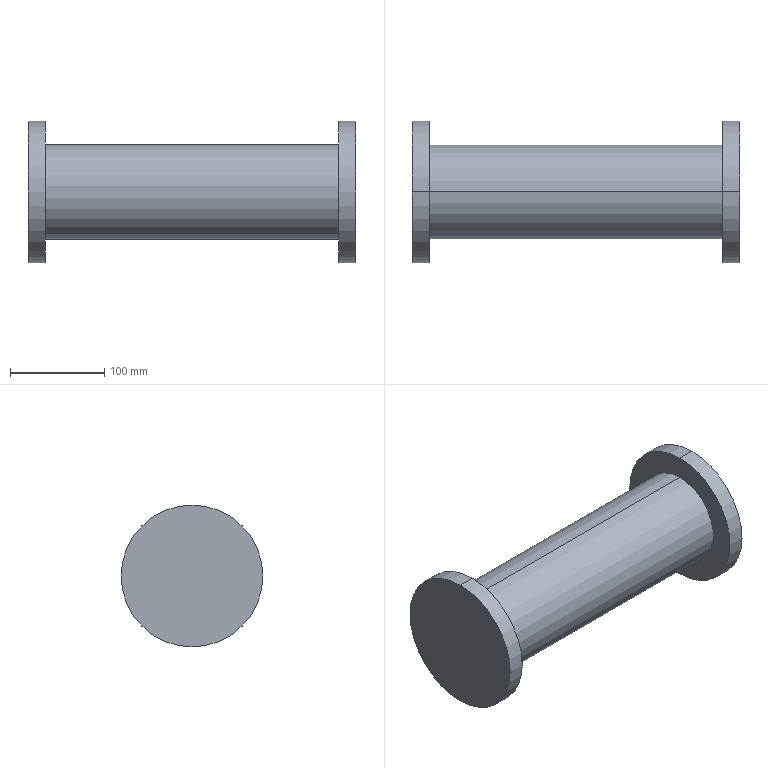Part | SolidWorks | features ICE 2, Extrusion 1 | 1 solid | 10 faces | box 347 x 150 x 150 mm | volume 3078761 mm3 | cylinder 6 | plane 4 | commonest cylinder face diameters 150 x4 100 x2
STEP:
#1=CARTESIAN_POINT('',(-329.,0.,-75.));
#2=VERTEX_POINT('',#1);
#3=CARTESIAN_POINT('',(-329.,0.,75.));
#4=VERTEX_POINT('',#3);
#5=CARTESIAN_POINT('',(-329.,0.,0.));
#6=DIRECTION('',(1.,0.,0.));
#7=DIRECTION('',(0.,0.,-1.));
#8=AXIS2_PLACEMENT_3D('',#5,#6,#7);
#9=CIRCLE('',#8,75.);
#10=EDGE_CURVE('',#2,#4,#9,.T.);
#11=ORIENTED_EDGE('',*,*,#10,.T.);
#12=CARTESIAN_POINT('',(-311.,0.,75.));
#13=VERTEX_POINT('',#12);
#14=CARTESIAN_POINT('',(-329.,0.,75.));
#15=DIRECTION('',(1.,0.,0.));
#16=VECTOR('',#15,1000.);
#17=LINE('',#14,#16);
#18=EDGE_CURVE('',#4,#13,#17,.T.);
#19=ORIENTED_EDGE('',*,*,#18,.T.);
#20=CARTESIAN_POINT('',(-311.,0.,-75.));
#21=VERTEX_POINT('',#20);
#22=CARTESIAN_POINT('',(-311.,0.,0.));
#23=DIRECTION('',(1.,0.,0.));
#24=DIRECTION('',(0.,0.,-1.));
#25=AXIS2_PLACEMENT_3D('',#22,#23,#24);
#26=CIRCLE('',#25,75.);
#27=EDGE_CURVE('',#21,#13,#26,.T.);
#28=ORIENTED_EDGE('',*,*,#27,.F.);
#29=CARTESIAN_POINT('',(-329.,0.,-75.));
#30=DIRECTION('',(1.,0.,0.));
#31=VECTOR('',#30,1000.);
#32=LINE('',#29,#31);
#33=EDGE_CURVE('',#2,#21,#32,.T.);
#34=ORIENTED_EDGE('',*,*,#33,.F.);
#35=EDGE_LOOP('',(#11,#19,#28,#34));
#36=FACE_OUTER_BOUND('',#35,.T.);
#37=CARTESIAN_POINT('',(-329.,0.,0.));
#38=DIRECTION('',(1.,0.,0.));
#39=DIRECTION('',(0.,0.,-1.));
#40=AXIS2_PLACEMENT_3D('',#37,#38,#39);
#41=CYLINDRICAL_SURFACE('',#40,75.);
#42=ADVANCED_FACE('',(#36),#41,.T.);
#43=CARTESIAN_POINT('',(-311.,0.,-50.));
#44=VERTEX_POINT('',#43);
#45=CARTESIAN_POINT('',(-311.,0.,50.));
#46=VERTEX_POINT('',#45);
#47=CARTESIAN_POINT('',(-311.,0.,0.));
#48=DIRECTION('',(1.,0.,0.));
#49=DIRECTION('',(0.,0.,-1.));
#50=AXIS2_PLACEMENT_3D('',#47,#48,#49);
#51=CIRCLE('',#50,50.);
#52=EDGE_CURVE('',#44,#46,#51,.T.);
#53=ORIENTED_EDGE('',*,*,#52,.T.);
#54=CARTESIAN_POINT('',(0.,0.,50.));
#55=VERTEX_POINT('',#54);
#56=CARTESIAN_POINT('',(-311.,0.,50.));
#57=DIRECTION('',(1.,0.,0.));
#58=VECTOR('',#57,1000.);
#59=LINE('',#56,#58);
#60=EDGE_CURVE('',#46,#55,#59,.T.);
#61=ORIENTED_EDGE('',*,*,#60,.T.);
#62=CARTESIAN_POINT('',(0.,0.,-50.));
#63=VERTEX_POINT('',#62);
#64=CARTESIAN_POINT('',(0.,0.,0.));
#65=DIRECTION('',(1.,0.,0.));
#66=DIRECTION('',(0.,0.,-1.));
#67=AXIS2_PLACEMENT_3D('',#64,#65,#66);
#68=CIRCLE('',#67,50.);
#69=EDGE_CURVE('',#63,#55,#68,.T.);
#70=ORIENTED_EDGE('',*,*,#69,.F.);
#71=CARTESIAN_POINT('',(-311.,0.,-50.));
#72=DIRECTION('',(1.,0.,0.));
#73=VECTOR('',#72,1000.);
#74=LINE('',#71,#73);
#75=EDGE_CURVE('',#44,#63,#74,.T.);
#76=ORIENTED_EDGE('',*,*,#75,.F.);
#77=EDGE_LOOP('',(#53,#61,#70,#76));
#78=FACE_OUTER_BOUND('',#77,.T.);
#79=CARTESIAN_POINT('',(-311.,0.,0.));
#80=DIRECTION('',(1.,0.,0.));
#81=DIRECTION('',(0.,0.,-1.));
#82=AXIS2_PLACEMENT_3D('',#79,#80,#81);
#83=CYLINDRICAL_SURFACE('',#82,50.);
#84=ADVANCED_FACE('',(#78),#83,.T.);
#85=CARTESIAN_POINT('',(18.,0.,-75.));
#86=VERTEX_POINT('',#85);
#87=CARTESIAN_POINT('',(18.,0.,75.));
#88=VERTEX_POINT('',#87);
#89=CARTESIAN_POINT('',(18.,0.,0.));
#90=DIRECTION('',(1.,0.,0.));
#91=DIRECTION('',(0.,0.,-1.));
#92=AXIS2_PLACEMENT_3D('',#89,#90,#91);
#93=CIRCLE('',#92,75.);
#94=EDGE_CURVE('',#86,#88,#93,.T.);
#95=ORIENTED_EDGE('',*,*,#94,.F.);
#96=CARTESIAN_POINT('',(0.,0.,-75.));
#97=VERTEX_POINT('',#96);
#98=CARTESIAN_POINT('',(18.,0.,-75.));
#99=DIRECTION('',(-1.,0.,0.));
#100=VECTOR('',#99,1000.);
#101=LINE('',#98,#100);
#102=EDGE_CURVE('',#86,#97,#101,.T.);
#103=ORIENTED_EDGE('',*,*,#102,.T.);
#104=CARTESIAN_POINT('',(0.,0.,75.));
#105=VERTEX_POINT('',#104);
#106=CARTESIAN_POINT('',(0.,0.,0.));
#107=DIRECTION('',(1.,0.,0.));
#108=DIRECTION('',(0.,0.,-1.));
#109=AXIS2_PLACEMENT_3D('',#106,#107,#108);
#110=CIRCLE('',#109,75.);
#111=EDGE_CURVE('',#97,#105,#110,.T.);
#112=ORIENTED_EDGE('',*,*,#111,.T.);
#113=CARTESIAN_POINT('',(18.,0.,75.));
#114=DIRECTION('',(-1.,0.,0.));
#115=VECTOR('',#114,1000.);
#116=LINE('',#113,#115);
#117=EDGE_CURVE('',#88,#105,#116,.T.);
#118=ORIENTED_EDGE('',*,*,#117,.F.);
#119=EDGE_LOOP('',(#95,#103,#112,#118));
#120=FACE_OUTER_BOUND('',#119,.T.);
#121=CARTESIAN_POINT('',(18.,0.,0.));
#122=DIRECTION('',(-1.,0.,0.));
#123=DIRECTION('',(0.,0.,1.));
#124=AXIS2_PLACEMENT_3D('',#121,#122,#123);
#125=CYLINDRICAL_SURFACE('',#124,75.);
#126=ADVANCED_FACE('',(#120),#125,.T.);
#127=ORIENTED_EDGE('',*,*,#102,.F.);
#128=CARTESIAN_POINT('',(18.,0.,0.));
#129=DIRECTION('',(1.,0.,0.));
#130=DIRECTION('',(0.,0.,-1.));
#131=AXIS2_PLACEMENT_3D('',#128,#129,#130);
#132=CIRCLE('',#131,75.);
#133=EDGE_CURVE('',#88,#86,#132,.T.);
#134=ORIENTED_EDGE('',*,*,#133,.F.);
#135=ORIENTED_EDGE('',*,*,#117,.T.);
#136=CARTESIAN_POINT('',(0.,0.,0.));
#137=DIRECTION('',(1.,0.,0.));
#138=DIRECTION('',(0.,0.,-1.));
#139=AXIS2_PLACEMENT_3D('',#136,#137,#138);
#140=CIRCLE('',#139,75.);
#141=EDGE_CURVE('',#105,#97,#140,.T.);
#142=ORIENTED_EDGE('',*,*,#141,.T.);
#143=EDGE_LOOP('',(#127,#134,#135,#142));
#144=FACE_OUTER_BOUND('',#143,.T.);
#145=CARTESIAN_POINT('',(18.,0.,0.));
#146=DIRECTION('',(-1.,0.,0.));
#147=DIRECTION('',(0.,0.,1.));
#148=AXIS2_PLACEMENT_3D('',#145,#146,#147);
#149=CYLINDRICAL_SURFACE('',#148,75.);
#150=ADVANCED_FACE('',(#144),#149,.T.);
#151=ORIENTED_EDGE('',*,*,#69,.T.);
#152=CARTESIAN_POINT('',(0.,0.,0.));
#153=DIRECTION('',(1.,0.,0.));
#154=DIRECTION('',(0.,0.,-1.));
#155=AXIS2_PLACEMENT_3D('',#152,#153,#154);
#156=CIRCLE('',#155,50.);
#157=EDGE_CURVE('',#55,#63,#156,.T.);
#158=ORIENTED_EDGE('',*,*,#157,.T.);
#159=EDGE_LOOP('',(#151,#158));
#160=FACE_BOUND('',#159,.T.);
#161=ORIENTED_EDGE('',*,*,#141,.F.);
#162=ORIENTED_EDGE('',*,*,#111,.F.);
#163=EDGE_LOOP('',(#161,#162));
#164=FACE_OUTER_BOUND('',#163,.T.);
#165=CARTESIAN_POINT('',(0.,0.,0.));
#166=DIRECTION('',(1.,0.,0.));
#167=DIRECTION('',(0.,0.,-1.));
#168=AXIS2_PLACEMENT_3D('',#165,#166,#167);
#169=PLANE('',#168);
#170=ADVANCED_FACE('',(#160,#164),#169,.F.);
#171=ORIENTED_EDGE('',*,*,#133,.T.);
#172=ORIENTED_EDGE('',*,*,#94,.T.);
#173=EDGE_LOOP('',(#171,#172));
#174=FACE_OUTER_BOUND('',#173,.T.);
#175=CARTESIAN_POINT('',(18.,0.,0.));
#176=DIRECTION('',(1.,0.,0.));
#177=DIRECTION('',(0.,0.,-1.));
#178=AXIS2_PLACEMENT_3D('',#175,#176,#177);
#179=PLANE('',#178);
#180=ADVANCED_FACE('',(#174),#179,.T.);
#181=ORIENTED_EDGE('',*,*,#60,.F.);
#182=CARTESIAN_POINT('',(-311.,0.,0.));
#183=DIRECTION('',(1.,0.,0.));
#184=DIRECTION('',(0.,0.,-1.));
#185=AXIS2_PLACEMENT_3D('',#182,#183,#184);
#186=CIRCLE('',#185,50.);
#187=EDGE_CURVE('',#46,#44,#186,.T.);
#188=ORIENTED_EDGE('',*,*,#187,.T.);
#189=ORIENTED_EDGE('',*,*,#75,.T.);
#190=ORIENTED_EDGE('',*,*,#157,.F.);
#191=EDGE_LOOP('',(#181,#188,#189,#190));
#192=FACE_OUTER_BOUND('',#191,.T.);
#193=CARTESIAN_POINT('',(-311.,0.,0.));
#194=DIRECTION('',(1.,0.,0.));
#195=DIRECTION('',(0.,0.,-1.));
#196=AXIS2_PLACEMENT_3D('',#193,#194,#195);
#197=CYLINDRICAL_SURFACE('',#196,50.);
#198=ADVANCED_FACE('',(#192),#197,.T.);
#199=ORIENTED_EDGE('',*,*,#18,.F.);
#200=CARTESIAN_POINT('',(-329.,0.,0.));
#201=DIRECTION('',(1.,0.,0.));
#202=DIRECTION('',(0.,0.,-1.));
#203=AXIS2_PLACEMENT_3D('',#200,#201,#202);
#204=CIRCLE('',#203,75.);
#205=EDGE_CURVE('',#4,#2,#204,.T.);
#206=ORIENTED_EDGE('',*,*,#205,.T.);
#207=ORIENTED_EDGE('',*,*,#33,.T.);
#208=CARTESIAN_POINT('',(-311.,0.,0.));
#209=DIRECTION('',(1.,0.,0.));
#210=DIRECTION('',(0.,0.,-1.));
#211=AXIS2_PLACEMENT_3D('',#208,#209,#210);
#212=CIRCLE('',#211,75.);
#213=EDGE_CURVE('',#13,#21,#212,.T.);
#214=ORIENTED_EDGE('',*,*,#213,.F.);
#215=EDGE_LOOP('',(#199,#206,#207,#214));
#216=FACE_OUTER_BOUND('',#215,.T.);
#217=CARTESIAN_POINT('',(-329.,0.,0.));
#218=DIRECTION('',(1.,0.,0.));
#219=DIRECTION('',(0.,0.,-1.));
#220=AXIS2_PLACEMENT_3D('',#217,#218,#219);
#221=CYLINDRICAL_SURFACE('',#220,75.);
#222=ADVANCED_FACE('',(#216),#221,.T.);
#223=ORIENTED_EDGE('',*,*,#10,.F.);
#224=ORIENTED_EDGE('',*,*,#205,.F.);
#225=EDGE_LOOP('',(#223,#224));
#226=FACE_OUTER_BOUND('',#225,.T.);
#227=CARTESIAN_POINT('',(-329.,0.,0.));
#228=DIRECTION('',(1.,0.,0.));
#229=DIRECTION('',(0.,0.,-1.));
#230=AXIS2_PLACEMENT_3D('',#227,#228,#229);
#231=PLANE('',#230);
#232=ADVANCED_FACE('',(#226),#231,.F.);
#233=ORIENTED_EDGE('',*,*,#52,.F.);
#234=ORIENTED_EDGE('',*,*,#187,.F.);
#235=EDGE_LOOP('',(#233,#234));
#236=FACE_BOUND('',#235,.T.);
#237=ORIENTED_EDGE('',*,*,#27,.T.);
#238=ORIENTED_EDGE('',*,*,#213,.T.);
#239=EDGE_LOOP('',(#237,#238));
#240=FACE_OUTER_BOUND('',#239,.T.);
#241=CARTESIAN_POINT('',(-311.,0.,0.));
#242=DIRECTION('',(1.,0.,0.));
#243=DIRECTION('',(0.,0.,-1.));
#244=AXIS2_PLACEMENT_3D('',#241,#242,#243);
#245=PLANE('',#244);
#246=ADVANCED_FACE('',(#236,#240),#245,.T.);
#247=CLOSED_SHELL('',(#42,#84,#126,#150,#170,#180,#198,#222,#232,#246));
#248=MANIFOLD_SOLID_BREP('',#247);
#249=CARTESIAN_POINT('',(0.,0.,0.));
#250=DIRECTION('',(0.,0.,1.));
#251=DIRECTION('',(1.,0.,0.));
#252=AXIS2_PLACEMENT_3D('',#249,#250,#251);
#253=(LENGTH_UNIT()NAMED_UNIT(*)SI_UNIT(.MILLI.,.METRE.));
#254=UNCERTAINTY_MEASURE_WITH_UNIT(LENGTH_MEASURE(0.00001),#253,'','');
#255=(NAMED_UNIT(*)PLANE_ANGLE_UNIT()SI_UNIT($,.RADIAN.));
#256=(NAMED_UNIT(*)SI_UNIT($,.STERADIAN.)SOLID_ANGLE_UNIT());
#257=(GEOMETRIC_REPRESENTATION_CONTEXT(3)GLOBAL_UNCERTAINTY_ASSIGNED_CONTEXT((#254))GLOBAL_UNIT_ASSIGNED_CONTEXT((#253,#255,#256))REPRESENTATION_CONTEXT('',''));
#258=ADVANCED_BREP_SHAPE_REPRESENTATION('',(#248,#252),#257);